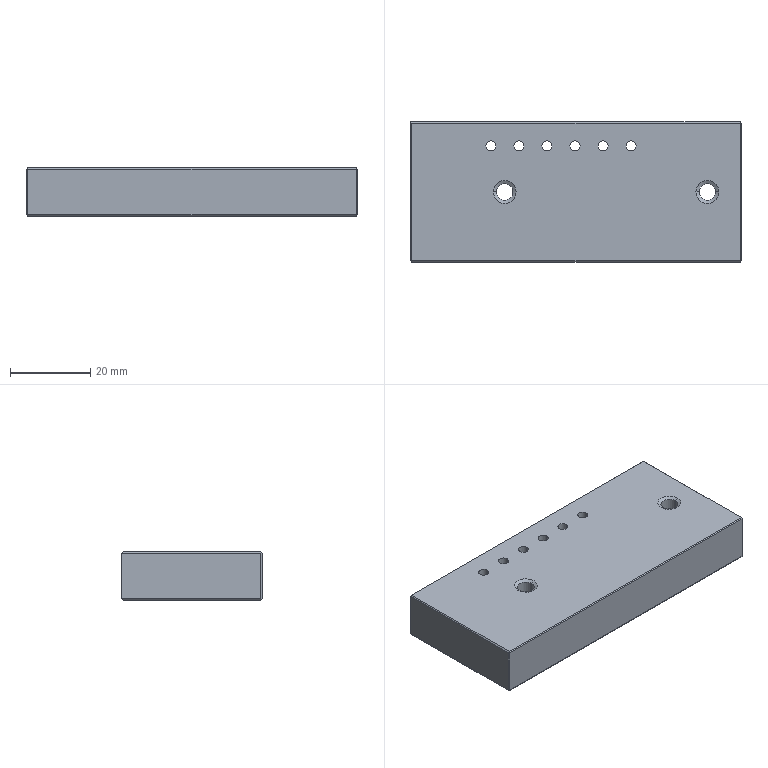Part | NX | 1 solid | 49 faces | box 82.5 x 35 x 12 mm | volume 33933 mm3 | plane 17 | cylinder 16 | cone 16 | commonest cylinder face diameters 2.5 x12 4.2 x4
STEP:
#1=CARTESIAN_POINT('',(-99.7,-60.,14.2));
#2=VERTEX_POINT('',#1);
#3=CARTESIAN_POINT('',(-99.7,-60.,2.8));
#4=VERTEX_POINT('',#3);
#5=CARTESIAN_POINT('',(-99.7,-60.,8.5));
#6=DIRECTION('',(0.,0.,-1.));
#7=VECTOR('',#6,1000.);
#8=LINE('',#5,#7);
#9=EDGE_CURVE('',#2,#4,#8,.T.);
#10=ORIENTED_EDGE('',*,*,#9,.T.);
#11=CARTESIAN_POINT('',(-17.8,-60.,2.8));
#12=VERTEX_POINT('',#11);
#13=CARTESIAN_POINT('',(0.,-60.,2.8));
#14=DIRECTION('',(-1.,0.,0.));
#15=VECTOR('',#14,1000.);
#16=LINE('',#13,#15);
#17=EDGE_CURVE('',#12,#4,#16,.T.);
#18=ORIENTED_EDGE('',*,*,#17,.F.);
#19=CARTESIAN_POINT('',(-17.8,-60.,14.2));
#20=VERTEX_POINT('',#19);
#21=CARTESIAN_POINT('',(-17.8,-60.,8.5));
#22=DIRECTION('',(0.,0.,1.));
#23=VECTOR('',#22,1000.);
#24=LINE('',#21,#23);
#25=EDGE_CURVE('',#12,#20,#24,.T.);
#26=ORIENTED_EDGE('',*,*,#25,.T.);
#27=CARTESIAN_POINT('',(0.,-60.,14.2));
#28=DIRECTION('',(1.,0.,0.));
#29=VECTOR('',#28,1000.);
#30=LINE('',#27,#29);
#31=EDGE_CURVE('',#2,#20,#30,.T.);
#32=ORIENTED_EDGE('',*,*,#31,.F.);
#33=EDGE_LOOP('',(#10,#18,#26,#32));
#34=FACE_BOUND('',#33,.T.);
#35=CARTESIAN_POINT('',(0.,-60.,0.));
#36=DIRECTION('',(0.,1.,0.));
#37=DIRECTION('',(1.,0.,0.));
#38=AXIS2_PLACEMENT_3D('',#35,#36,#37);
#39=PLANE('',#38);
#40=ADVANCED_FACE('',(#34),#39,.F.);
#41=CARTESIAN_POINT('',(-100.,-25.,2.8));
#42=VERTEX_POINT('',#41);
#43=CARTESIAN_POINT('',(-100.,-25.,14.2));
#44=VERTEX_POINT('',#43);
#45=CARTESIAN_POINT('',(-100.,-25.,0.));
#46=DIRECTION('',(0.,0.,1.));
#47=VECTOR('',#46,1000.);
#48=LINE('',#45,#47);
#49=EDGE_CURVE('',#42,#44,#48,.T.);
#50=ORIENTED_EDGE('',*,*,#49,.F.);
#51=CARTESIAN_POINT('',(-100.,-59.7,2.8));
#52=VERTEX_POINT('',#51);
#53=CARTESIAN_POINT('',(-100.,-42.5,2.8));
#54=DIRECTION('',(0.,1.,0.));
#55=VECTOR('',#54,1000.);
#56=LINE('',#53,#55);
#57=EDGE_CURVE('',#52,#42,#56,.T.);
#58=ORIENTED_EDGE('',*,*,#57,.F.);
#59=CARTESIAN_POINT('',(-100.,-59.7,14.2));
#60=VERTEX_POINT('',#59);
#61=CARTESIAN_POINT('',(-100.,-59.7,8.5));
#62=DIRECTION('',(0.,0.,-1.));
#63=VECTOR('',#62,1000.);
#64=LINE('',#61,#63);
#65=EDGE_CURVE('',#60,#52,#64,.T.);
#66=ORIENTED_EDGE('',*,*,#65,.F.);
#67=CARTESIAN_POINT('',(-100.,-42.5,14.2));
#68=DIRECTION('',(0.,-1.,0.));
#69=VECTOR('',#68,1000.);
#70=LINE('',#67,#69);
#71=EDGE_CURVE('',#44,#60,#70,.T.);
#72=ORIENTED_EDGE('',*,*,#71,.F.);
#73=EDGE_LOOP('',(#50,#58,#66,#72));
#74=FACE_BOUND('',#73,.T.);
#75=CARTESIAN_POINT('',(-100.,0.,0.));
#76=DIRECTION('',(1.,0.,0.));
#77=DIRECTION('',(0.,1.,0.));
#78=AXIS2_PLACEMENT_3D('',#75,#76,#77);
#79=PLANE('',#78);
#80=ADVANCED_FACE('',(#74),#79,.F.);
#81=CARTESIAN_POINT('',(-17.8,-25.,2.8));
#82=VERTEX_POINT('',#81);
#83=CARTESIAN_POINT('',(-17.8,-25.,14.2));
#84=VERTEX_POINT('',#83);
#85=CARTESIAN_POINT('',(-17.8,-25.,8.5));
#86=DIRECTION('',(0.,0.,1.));
#87=VECTOR('',#86,1000.);
#88=LINE('',#85,#87);
#89=EDGE_CURVE('',#82,#84,#88,.T.);
#90=ORIENTED_EDGE('',*,*,#89,.F.);
#91=CARTESIAN_POINT('',(0.,-25.,2.8));
#92=DIRECTION('',(1.,0.,0.));
#93=VECTOR('',#92,1000.);
#94=LINE('',#91,#93);
#95=EDGE_CURVE('',#42,#82,#94,.T.);
#96=ORIENTED_EDGE('',*,*,#95,.F.);
#97=ORIENTED_EDGE('',*,*,#49,.T.);
#98=CARTESIAN_POINT('',(0.,-25.,14.2));
#99=DIRECTION('',(1.,0.,0.));
#100=VECTOR('',#99,1000.);
#101=LINE('',#98,#100);
#102=EDGE_CURVE('',#44,#84,#101,.T.);
#103=ORIENTED_EDGE('',*,*,#102,.T.);
#104=EDGE_LOOP('',(#90,#96,#97,#103));
#105=FACE_BOUND('',#104,.T.);
#106=CARTESIAN_POINT('',(-8.5,-25.,1.2));
#107=DIRECTION('',(0.,-1.,0.));
#108=DIRECTION('',(-1.,0.,0.));
#109=AXIS2_PLACEMENT_3D('',#106,#107,#108);
#110=PLANE('',#109);
#111=ADVANCED_FACE('',(#105),#110,.F.);
#112=CARTESIAN_POINT('',(-17.8,-59.7,14.5));
#113=VERTEX_POINT('',#112);
#114=CARTESIAN_POINT('',(-99.7,-59.7,14.5));
#115=VERTEX_POINT('',#114);
#116=CARTESIAN_POINT('',(0.,-59.7,14.5));
#117=DIRECTION('',(-1.,0.,0.));
#118=VECTOR('',#117,1000.);
#119=LINE('',#116,#118);
#120=EDGE_CURVE('',#113,#115,#119,.T.);
#121=ORIENTED_EDGE('',*,*,#120,.T.);
#122=CARTESIAN_POINT('',(-99.85,-59.85,14.35));
#123=VERTEX_POINT('',#122);
#124=CARTESIAN_POINT('',(-114.2,-74.2,0.));
#125=DIRECTION('',(-0.5774,-0.5774,-0.5774));
#126=VECTOR('',#125,1000.);
#127=LINE('',#124,#126);
#128=EDGE_CURVE('',#115,#123,#127,.T.);
#129=ORIENTED_EDGE('',*,*,#128,.T.);
#130=CARTESIAN_POINT('',(-85.5,-74.2,0.));
#131=DIRECTION('',(0.5774,-0.5774,-0.5774));
#132=VECTOR('',#131,1000.);
#133=LINE('',#130,#132);
#134=EDGE_CURVE('',#123,#2,#133,.T.);
#135=ORIENTED_EDGE('',*,*,#134,.T.);
#136=ORIENTED_EDGE('',*,*,#31,.T.);
#137=CARTESIAN_POINT('',(-17.65,-59.85,14.35));
#138=VERTEX_POINT('',#137);
#139=CARTESIAN_POINT('',(-32.,-74.2,0.));
#140=DIRECTION('',(0.5774,0.5774,0.5774));
#141=VECTOR('',#140,1000.);
#142=LINE('',#139,#141);
#143=EDGE_CURVE('',#20,#138,#142,.T.);
#144=ORIENTED_EDGE('',*,*,#143,.T.);
#145=CARTESIAN_POINT('',(-3.3,-74.2,0.));
#146=DIRECTION('',(-0.5774,0.5774,0.5774));
#147=VECTOR('',#146,1000.);
#148=LINE('',#145,#147);
#149=EDGE_CURVE('',#138,#113,#148,.T.);
#150=ORIENTED_EDGE('',*,*,#149,.T.);
#151=EDGE_LOOP('',(#121,#129,#135,#136,#144,#150));
#152=FACE_BOUND('',#151,.T.);
#153=CARTESIAN_POINT('',(-51.25,-59.85,14.35));
#154=DIRECTION('',(0.,0.7071,-0.7071));
#155=DIRECTION('',(-1.,0.,0.));
#156=AXIS2_PLACEMENT_3D('',#153,#154,#155);
#157=PLANE('',#156);
#158=ADVANCED_FACE('',(#152),#157,.F.);
#159=CARTESIAN_POINT('',(-17.5,-25.3,14.2));
#160=VERTEX_POINT('',#159);
#161=CARTESIAN_POINT('',(-17.5,-59.7,14.2));
#162=VERTEX_POINT('',#161);
#163=CARTESIAN_POINT('',(-17.5,-42.5,14.2));
#164=DIRECTION('',(0.,-1.,0.));
#165=VECTOR('',#164,1000.);
#166=LINE('',#163,#165);
#167=EDGE_CURVE('',#160,#162,#166,.T.);
#168=ORIENTED_EDGE('',*,*,#167,.T.);
#169=CARTESIAN_POINT('',(-17.5,-59.7,2.8));
#170=VERTEX_POINT('',#169);
#171=CARTESIAN_POINT('',(-17.5,-59.7,8.5));
#172=DIRECTION('',(0.,0.,1.));
#173=VECTOR('',#172,1000.);
#174=LINE('',#171,#173);
#175=EDGE_CURVE('',#170,#162,#174,.T.);
#176=ORIENTED_EDGE('',*,*,#175,.F.);
#177=CARTESIAN_POINT('',(-17.5,-25.3,2.8));
#178=VERTEX_POINT('',#177);
#179=CARTESIAN_POINT('',(-17.5,-42.5,2.8));
#180=DIRECTION('',(0.,1.,0.));
#181=VECTOR('',#180,1000.);
#182=LINE('',#179,#181);
#183=EDGE_CURVE('',#170,#178,#182,.T.);
#184=ORIENTED_EDGE('',*,*,#183,.T.);
#185=CARTESIAN_POINT('',(-17.5,-25.3,8.5));
#186=DIRECTION('',(0.,0.,1.));
#187=VECTOR('',#186,1000.);
#188=LINE('',#185,#187);
#189=EDGE_CURVE('',#178,#160,#188,.T.);
#190=ORIENTED_EDGE('',*,*,#189,.T.);
#191=EDGE_LOOP('',(#168,#176,#184,#190));
#192=FACE_BOUND('',#191,.T.);
#193=CARTESIAN_POINT('',(-17.5,-38.5,5.));
#194=DIRECTION('',(1.,0.,0.));
#195=DIRECTION('',(0.,1.,0.));
#196=AXIS2_PLACEMENT_3D('',#193,#194,#195);
#197=PLANE('',#196);
#198=ADVANCED_FACE('',(#192),#197,.T.);
#199=CARTESIAN_POINT('',(-99.7,-25.3,14.5));
#200=VERTEX_POINT('',#199);
#201=CARTESIAN_POINT('',(-99.7,0.,14.5));
#202=DIRECTION('',(0.,-1.,0.));
#203=VECTOR('',#202,1000.);
#204=LINE('',#201,#203);
#205=EDGE_CURVE('',#200,#115,#204,.T.);
#206=ORIENTED_EDGE('',*,*,#205,.T.);
#207=ORIENTED_EDGE('',*,*,#120,.F.);
#208=CARTESIAN_POINT('',(-17.8,-25.3,14.5));
#209=VERTEX_POINT('',#208);
#210=CARTESIAN_POINT('',(-17.8,0.,14.5));
#211=DIRECTION('',(0.,1.,0.));
#212=VECTOR('',#211,1000.);
#213=LINE('',#210,#212);
#214=EDGE_CURVE('',#113,#209,#213,.T.);
#215=ORIENTED_EDGE('',*,*,#214,.T.);
#216=CARTESIAN_POINT('',(0.,-25.3,14.5));
#217=DIRECTION('',(1.,0.,0.));
#218=VECTOR('',#217,1000.);
#219=LINE('',#216,#218);
#220=EDGE_CURVE('',#200,#209,#219,.T.);
#221=ORIENTED_EDGE('',*,*,#220,.F.);
#222=EDGE_LOOP('',(#206,#207,#215,#221));
#223=FACE_BOUND('',#222,.T.);
#224=CARTESIAN_POINT('',(-28.797,-42.5,14.5));
#225=VERTEX_POINT('',#224);
#226=CARTESIAN_POINT('',(-23.077,-42.5,14.5));
#227=VERTEX_POINT('',#226);
#228=CARTESIAN_POINT('',(-25.937,-42.5,14.5));
#229=DIRECTION('',(0.,0.,1.));
#230=DIRECTION('',(1.,0.,0.));
#231=AXIS2_PLACEMENT_3D('',#228,#229,#230);
#232=CIRCLE('',#231,2.86);
#233=EDGE_CURVE('',#225,#227,#232,.T.);
#234=ORIENTED_EDGE('',*,*,#233,.F.);
#235=CARTESIAN_POINT('',(-25.937,-42.5,14.5));
#236=DIRECTION('',(0.,0.,1.));
#237=DIRECTION('',(1.,0.,0.));
#238=AXIS2_PLACEMENT_3D('',#235,#236,#237);
#239=CIRCLE('',#238,2.86);
#240=EDGE_CURVE('',#227,#225,#239,.T.);
#241=ORIENTED_EDGE('',*,*,#240,.F.);
#242=EDGE_LOOP('',(#234,#241));
#243=FACE_BOUND('',#242,.T.);
#244=CARTESIAN_POINT('',(-79.422,-42.5,14.5));
#245=VERTEX_POINT('',#244);
#246=CARTESIAN_POINT('',(-73.702,-42.5,14.5));
#247=VERTEX_POINT('',#246);
#248=CARTESIAN_POINT('',(-76.562,-42.5,14.5));
#249=DIRECTION('',(0.,0.,1.));
#250=DIRECTION('',(1.,0.,0.));
#251=AXIS2_PLACEMENT_3D('',#248,#249,#250);
#252=CIRCLE('',#251,2.86);
#253=EDGE_CURVE('',#245,#247,#252,.T.);
#254=ORIENTED_EDGE('',*,*,#253,.F.);
#255=CARTESIAN_POINT('',(-76.562,-42.5,14.5));
#256=DIRECTION('',(0.,0.,1.));
#257=DIRECTION('',(1.,0.,0.));
#258=AXIS2_PLACEMENT_3D('',#255,#256,#257);
#259=CIRCLE('',#258,2.86);
#260=EDGE_CURVE('',#247,#245,#259,.T.);
#261=ORIENTED_EDGE('',*,*,#260,.F.);
#262=EDGE_LOOP('',(#254,#261));
#263=FACE_BOUND('',#262,.T.);
#264=CARTESIAN_POINT('',(-43.75,-31.,14.5));
#265=VERTEX_POINT('',#264);
#266=CARTESIAN_POINT('',(-46.25,-31.,14.5));
#267=VERTEX_POINT('',#266);
#268=CARTESIAN_POINT('',(-45.,-31.,14.5));
#269=DIRECTION('',(0.,0.,-1.));
#270=DIRECTION('',(-1.,0.,0.));
#271=AXIS2_PLACEMENT_3D('',#268,#269,#270);
#272=CIRCLE('',#271,1.25);
#273=EDGE_CURVE('',#265,#267,#272,.T.);
#274=ORIENTED_EDGE('',*,*,#273,.T.);
#275=CARTESIAN_POINT('',(-45.,-31.,14.5));
#276=DIRECTION('',(0.,0.,-1.));
#277=DIRECTION('',(-1.,0.,0.));
#278=AXIS2_PLACEMENT_3D('',#275,#276,#277);
#279=CIRCLE('',#278,1.25);
#280=EDGE_CURVE('',#267,#265,#279,.T.);
#281=ORIENTED_EDGE('',*,*,#280,.T.);
#282=EDGE_LOOP('',(#274,#281));
#283=FACE_BOUND('',#282,.T.);
#284=CARTESIAN_POINT('',(-50.75,-31.,14.5));
#285=VERTEX_POINT('',#284);
#286=CARTESIAN_POINT('',(-53.25,-31.,14.5));
#287=VERTEX_POINT('',#286);
#288=CARTESIAN_POINT('',(-52.,-31.,14.5));
#289=DIRECTION('',(0.,0.,-1.));
#290=DIRECTION('',(-1.,0.,0.));
#291=AXIS2_PLACEMENT_3D('',#288,#289,#290);
#292=CIRCLE('',#291,1.25);
#293=EDGE_CURVE('',#285,#287,#292,.T.);
#294=ORIENTED_EDGE('',*,*,#293,.T.);
#295=CARTESIAN_POINT('',(-52.,-31.,14.5));
#296=DIRECTION('',(0.,0.,-1.));
#297=DIRECTION('',(-1.,0.,0.));
#298=AXIS2_PLACEMENT_3D('',#295,#296,#297);
#299=CIRCLE('',#298,1.25);
#300=EDGE_CURVE('',#287,#285,#299,.T.);
#301=ORIENTED_EDGE('',*,*,#300,.T.);
#302=EDGE_LOOP('',(#294,#301));
#303=FACE_BOUND('',#302,.T.);
#304=CARTESIAN_POINT('',(-57.75,-31.,14.5));
#305=VERTEX_POINT('',#304);
#306=CARTESIAN_POINT('',(-60.25,-31.,14.5));
#307=VERTEX_POINT('',#306);
#308=CARTESIAN_POINT('',(-59.,-31.,14.5));
#309=DIRECTION('',(0.,0.,-1.));
#310=DIRECTION('',(-1.,0.,0.));
#311=AXIS2_PLACEMENT_3D('',#308,#309,#310);
#312=CIRCLE('',#311,1.25);
#313=EDGE_CURVE('',#305,#307,#312,.T.);
#314=ORIENTED_EDGE('',*,*,#313,.T.);
#315=CARTESIAN_POINT('',(-59.,-31.,14.5));
#316=DIRECTION('',(0.,0.,-1.));
#317=DIRECTION('',(-1.,0.,0.));
#318=AXIS2_PLACEMENT_3D('',#315,#316,#317);
#319=CIRCLE('',#318,1.25);
#320=EDGE_CURVE('',#307,#305,#319,.T.);
#321=ORIENTED_EDGE('',*,*,#320,.T.);
#322=EDGE_LOOP('',(#314,#321));
#323=FACE_BOUND('',#322,.T.);
#324=CARTESIAN_POINT('',(-64.75,-31.,14.5));
#325=VERTEX_POINT('',#324);
#326=CARTESIAN_POINT('',(-67.25,-31.,14.5));
#327=VERTEX_POINT('',#326);
#328=CARTESIAN_POINT('',(-66.,-31.,14.5));
#329=DIRECTION('',(0.,0.,-1.));
#330=DIRECTION('',(-1.,0.,0.));
#331=AXIS2_PLACEMENT_3D('',#328,#329,#330);
#332=CIRCLE('',#331,1.25);
#333=EDGE_CURVE('',#325,#327,#332,.T.);
#334=ORIENTED_EDGE('',*,*,#333,.T.);
#335=CARTESIAN_POINT('',(-66.,-31.,14.5));
#336=DIRECTION('',(0.,0.,-1.));
#337=DIRECTION('',(-1.,0.,0.));
#338=AXIS2_PLACEMENT_3D('',#335,#336,#337);
#339=CIRCLE('',#338,1.25);
#340=EDGE_CURVE('',#327,#325,#339,.T.);
#341=ORIENTED_EDGE('',*,*,#340,.T.);
#342=EDGE_LOOP('',(#334,#341));
#343=FACE_BOUND('',#342,.T.);
#344=CARTESIAN_POINT('',(-71.75,-31.,14.5));
#345=VERTEX_POINT('',#344);
#346=CARTESIAN_POINT('',(-74.25,-31.,14.5));
#347=VERTEX_POINT('',#346);
#348=CARTESIAN_POINT('',(-73.,-31.,14.5));
#349=DIRECTION('',(0.,0.,-1.));
#350=DIRECTION('',(-1.,0.,0.));
#351=AXIS2_PLACEMENT_3D('',#348,#349,#350);
#352=CIRCLE('',#351,1.25);
#353=EDGE_CURVE('',#345,#347,#352,.T.);
#354=ORIENTED_EDGE('',*,*,#353,.T.);
#355=CARTESIAN_POINT('',(-73.,-31.,14.5));
#356=DIRECTION('',(0.,0.,-1.));
#357=DIRECTION('',(-1.,0.,0.));
#358=AXIS2_PLACEMENT_3D('',#355,#356,#357);
#359=CIRCLE('',#358,1.25);
#360=EDGE_CURVE('',#347,#345,#359,.T.);
#361=ORIENTED_EDGE('',*,*,#360,.T.);
#362=EDGE_LOOP('',(#354,#361));
#363=FACE_BOUND('',#362,.T.);
#364=CARTESIAN_POINT('',(-78.75,-31.,14.5));
#365=VERTEX_POINT('',#364);
#366=CARTESIAN_POINT('',(-81.25,-31.,14.5));
#367=VERTEX_POINT('',#366);
#368=CARTESIAN_POINT('',(-80.,-31.,14.5));
#369=DIRECTION('',(0.,0.,-1.));
#370=DIRECTION('',(-1.,0.,0.));
#371=AXIS2_PLACEMENT_3D('',#368,#369,#370);
#372=CIRCLE('',#371,1.25);
#373=EDGE_CURVE('',#365,#367,#372,.T.);
#374=ORIENTED_EDGE('',*,*,#373,.T.);
#375=CARTESIAN_POINT('',(-80.,-31.,14.5));
#376=DIRECTION('',(0.,0.,-1.));
#377=DIRECTION('',(-1.,0.,0.));
#378=AXIS2_PLACEMENT_3D('',#375,#376,#377);
#379=CIRCLE('',#378,1.25);
#380=EDGE_CURVE('',#367,#365,#379,.T.);
#381=ORIENTED_EDGE('',*,*,#380,.T.);
#382=EDGE_LOOP('',(#374,#381));
#383=FACE_BOUND('',#382,.T.);
#384=CARTESIAN_POINT('',(-20.5,7.5,14.5));
#385=DIRECTION('',(0.,0.,-1.));
#386=DIRECTION('',(0.,-1.,0.));
#387=AXIS2_PLACEMENT_3D('',#384,#385,#386);
#388=PLANE('',#387);
#389=ADVANCED_FACE('',(#223,#243,#263,#283,#303,#323,#343,#363,#383),#388,.F.);
#390=ORIENTED_EDGE('',*,*,#9,.F.);
#391=ORIENTED_EDGE('',*,*,#134,.F.);
#392=CARTESIAN_POINT('',(-114.2,-45.5,0.));
#393=DIRECTION('',(0.5774,-0.5774,0.5774));
#394=VECTOR('',#393,1000.);
#395=LINE('',#392,#394);
#396=EDGE_CURVE('',#60,#123,#395,.T.);
#397=ORIENTED_EDGE('',*,*,#396,.F.);
#398=ORIENTED_EDGE('',*,*,#65,.T.);
#399=CARTESIAN_POINT('',(-99.85,-59.85,2.65));
#400=VERTEX_POINT('',#399);
#401=CARTESIAN_POINT('',(-97.2,-62.5,0.));
#402=DIRECTION('',(0.5774,-0.5774,-0.5774));
#403=VECTOR('',#402,1000.);
#404=LINE('',#401,#403);
#405=EDGE_CURVE('',#52,#400,#404,.T.);
#406=ORIENTED_EDGE('',*,*,#405,.T.);
#407=CARTESIAN_POINT('',(-102.5,-57.2,0.));
#408=DIRECTION('',(-0.5774,0.5774,-0.5774));
#409=VECTOR('',#408,1000.);
#410=LINE('',#407,#409);
#411=EDGE_CURVE('',#4,#400,#410,.T.);
#412=ORIENTED_EDGE('',*,*,#411,.F.);
#413=EDGE_LOOP('',(#390,#391,#397,#398,#406,#412));
#414=FACE_BOUND('',#413,.T.);
#415=CARTESIAN_POINT('',(-99.85,-59.85,8.5));
#416=DIRECTION('',(-0.7071,-0.7071,0.));
#417=DIRECTION('',(-0.7071,0.7071,0.));
#418=AXIS2_PLACEMENT_3D('',#415,#416,#417);
#419=PLANE('',#418);
#420=ADVANCED_FACE('',(#414),#419,.T.);
#421=CARTESIAN_POINT('',(-17.8,-59.7,2.5));
#422=VERTEX_POINT('',#421);
#423=CARTESIAN_POINT('',(-17.8,-25.3,2.5));
#424=VERTEX_POINT('',#423);
#425=CARTESIAN_POINT('',(-17.8,0.,2.5));
#426=DIRECTION('',(0.,1.,0.));
#427=VECTOR('',#426,1000.);
#428=LINE('',#425,#427);
#429=EDGE_CURVE('',#422,#424,#428,.T.);
#430=ORIENTED_EDGE('',*,*,#429,.T.);
#431=CARTESIAN_POINT('',(-17.65,-25.15,2.65));
#432=VERTEX_POINT('',#431);
#433=CARTESIAN_POINT('',(0.,-7.5,20.3));
#434=DIRECTION('',(-0.5774,-0.5774,-0.5774));
#435=VECTOR('',#434,1000.);
#436=LINE('',#433,#435);
#437=EDGE_CURVE('',#432,#424,#436,.T.);
#438=ORIENTED_EDGE('',*,*,#437,.F.);
#439=CARTESIAN_POINT('',(-42.8,0.,-22.5));
#440=DIRECTION('',(0.5774,-0.5774,0.5774));
#441=VECTOR('',#440,1000.);
#442=LINE('',#439,#441);
#443=EDGE_CURVE('',#432,#178,#442,.T.);
#444=ORIENTED_EDGE('',*,*,#443,.T.);
#445=ORIENTED_EDGE('',*,*,#183,.F.);
#446=CARTESIAN_POINT('',(-17.65,-59.85,2.65));
#447=VERTEX_POINT('',#446);
#448=CARTESIAN_POINT('',(0.,-42.2,20.3));
#449=DIRECTION('',(0.5774,0.5774,0.5774));
#450=VECTOR('',#449,1000.);
#451=LINE('',#448,#450);
#452=EDGE_CURVE('',#447,#170,#451,.T.);
#453=ORIENTED_EDGE('',*,*,#452,.F.);
#454=CARTESIAN_POINT('',(0.,-77.5,20.3));
#455=DIRECTION('',(-0.5774,0.5774,-0.5774));
#456=VECTOR('',#455,1000.);
#457=LINE('',#454,#456);
#458=EDGE_CURVE('',#447,#422,#457,.T.);
#459=ORIENTED_EDGE('',*,*,#458,.T.);
#460=EDGE_LOOP('',(#430,#438,#444,#445,#453,#459));
#461=FACE_BOUND('',#460,.T.);
#462=CARTESIAN_POINT('',(-17.65,-42.5,2.65));
#463=DIRECTION('',(-0.7071,0.,0.7071));
#464=DIRECTION('',(0.,1.,0.));
#465=AXIS2_PLACEMENT_3D('',#462,#463,#464);
#466=PLANE('',#465);
#467=ADVANCED_FACE('',(#461),#466,.F.);
#468=CARTESIAN_POINT('',(-99.7,-25.3,2.5));
#469=VERTEX_POINT('',#468);
#470=CARTESIAN_POINT('',(0.,-25.3,2.5));
#471=DIRECTION('',(1.,0.,0.));
#472=VECTOR('',#471,1000.);
#473=LINE('',#470,#472);
#474=EDGE_CURVE('',#469,#424,#473,.T.);
#475=ORIENTED_EDGE('',*,*,#474,.T.);
#476=ORIENTED_EDGE('',*,*,#429,.F.);
#477=CARTESIAN_POINT('',(-99.7,-59.7,2.5));
#478=VERTEX_POINT('',#477);
#479=CARTESIAN_POINT('',(0.,-59.7,2.5));
#480=DIRECTION('',(1.,0.,0.));
#481=VECTOR('',#480,1000.);
#482=LINE('',#479,#481);
#483=EDGE_CURVE('',#478,#422,#482,.T.);
#484=ORIENTED_EDGE('',*,*,#483,.F.);
#485=CARTESIAN_POINT('',(-99.7,0.,2.5));
#486=DIRECTION('',(0.,1.,0.));
#487=VECTOR('',#486,1000.);
#488=LINE('',#485,#487);
#489=EDGE_CURVE('',#478,#469,#488,.T.);
#490=ORIENTED_EDGE('',*,*,#489,.T.);
#491=EDGE_LOOP('',(#475,#476,#484,#490));
#492=FACE_BOUND('',#491,.T.);
#493=CARTESIAN_POINT('',(-28.037,-42.5,2.5));
#494=VERTEX_POINT('',#493);
#495=CARTESIAN_POINT('',(-23.837,-42.5,2.5));
#496=VERTEX_POINT('',#495);
#497=CARTESIAN_POINT('',(-25.937,-42.5,2.5));
#498=DIRECTION('',(0.,0.,1.));
#499=DIRECTION('',(1.,0.,0.));
#500=AXIS2_PLACEMENT_3D('',#497,#498,#499);
#501=CIRCLE('',#500,2.1);
#502=EDGE_CURVE('',#494,#496,#501,.T.);
#503=ORIENTED_EDGE('',*,*,#502,.T.);
#504=CARTESIAN_POINT('',(-25.937,-42.5,2.5));
#505=DIRECTION('',(0.,0.,1.));
#506=DIRECTION('',(1.,0.,0.));
#507=AXIS2_PLACEMENT_3D('',#504,#505,#506);
#508=CIRCLE('',#507,2.1);
#509=EDGE_CURVE('',#496,#494,#508,.T.);
#510=ORIENTED_EDGE('',*,*,#509,.T.);
#511=EDGE_LOOP('',(#503,#510));
#512=FACE_BOUND('',#511,.T.);
#513=CARTESIAN_POINT('',(-78.3,-31.,2.5));
#514=VERTEX_POINT('',#513);
#515=CARTESIAN_POINT('',(-81.7,-31.,2.5));
#516=VERTEX_POINT('',#515);
#517=CARTESIAN_POINT('',(-80.,-31.,2.5));
#518=DIRECTION('',(0.,0.,-1.));
#519=DIRECTION('',(-1.,0.,0.));
#520=AXIS2_PLACEMENT_3D('',#517,#518,#519);
#521=CIRCLE('',#520,1.7);
#522=EDGE_CURVE('',#514,#516,#521,.T.);
#523=ORIENTED_EDGE('',*,*,#522,.F.);
#524=CARTESIAN_POINT('',(-80.,-31.,2.5));
#525=DIRECTION('',(0.,0.,-1.));
#526=DIRECTION('',(-1.,0.,0.));
#527=AXIS2_PLACEMENT_3D('',#524,#525,#526);
#528=CIRCLE('',#527,1.7);
#529=EDGE_CURVE('',#516,#514,#528,.T.);
#530=ORIENTED_EDGE('',*,*,#529,.F.);
#531=EDGE_LOOP('',(#523,#530));
#532=FACE_BOUND('',#531,.T.);
#533=CARTESIAN_POINT('',(-64.3,-31.,2.5));
#534=VERTEX_POINT('',#533);
#535=CARTESIAN_POINT('',(-67.7,-31.,2.5));
#536=VERTEX_POINT('',#535);
#537=CARTESIAN_POINT('',(-66.,-31.,2.5));
#538=DIRECTION('',(0.,0.,-1.));
#539=DIRECTION('',(-1.,0.,0.));
#540=AXIS2_PLACEMENT_3D('',#537,#538,#539);
#541=CIRCLE('',#540,1.7);
#542=EDGE_CURVE('',#534,#536,#541,.T.);
#543=ORIENTED_EDGE('',*,*,#542,.F.);
#544=CARTESIAN_POINT('',(-66.,-31.,2.5));
#545=DIRECTION('',(0.,0.,-1.));
#546=DIRECTION('',(-1.,0.,0.));
#547=AXIS2_PLACEMENT_3D('',#544,#545,#546);
#548=CIRCLE('',#547,1.7);
#549=EDGE_CURVE('',#536,#534,#548,.T.);
#550=ORIENTED_EDGE('',*,*,#549,.F.);
#551=EDGE_LOOP('',(#543,#550));
#552=FACE_BOUND('',#551,.T.);
#553=CARTESIAN_POINT('',(-50.3,-31.,2.5));
#554=VERTEX_POINT('',#553);
#555=CARTESIAN_POINT('',(-53.7,-31.,2.5));
#556=VERTEX_POINT('',#555);
#557=CARTESIAN_POINT('',(-52.,-31.,2.5));
#558=DIRECTION('',(0.,0.,-1.));
#559=DIRECTION('',(-1.,0.,0.));
#560=AXIS2_PLACEMENT_3D('',#557,#558,#559);
#561=CIRCLE('',#560,1.7);
#562=EDGE_CURVE('',#554,#556,#561,.T.);
#563=ORIENTED_EDGE('',*,*,#562,.F.);
#564=CARTESIAN_POINT('',(-52.,-31.,2.5));
#565=DIRECTION('',(0.,0.,-1.));
#566=DIRECTION('',(-1.,0.,0.));
#567=AXIS2_PLACEMENT_3D('',#564,#565,#566);
#568=CIRCLE('',#567,1.7);
#569=EDGE_CURVE('',#556,#554,#568,.T.);
#570=ORIENTED_EDGE('',*,*,#569,.F.);
#571=EDGE_LOOP('',(#563,#570));
#572=FACE_BOUND('',#571,.T.);
#573=CARTESIAN_POINT('',(-78.662,-42.5,2.5));
#574=VERTEX_POINT('',#573);
#575=CARTESIAN_POINT('',(-74.462,-42.5,2.5));
#576=VERTEX_POINT('',#575);
#577=CARTESIAN_POINT('',(-76.562,-42.5,2.5));
#578=DIRECTION('',(0.,0.,1.));
#579=DIRECTION('',(1.,0.,0.));
#580=AXIS2_PLACEMENT_3D('',#577,#578,#579);
#581=CIRCLE('',#580,2.1);
#582=EDGE_CURVE('',#574,#576,#581,.T.);
#583=ORIENTED_EDGE('',*,*,#582,.T.);
#584=CARTESIAN_POINT('',(-76.562,-42.5,2.5));
#585=DIRECTION('',(0.,0.,1.));
#586=DIRECTION('',(1.,0.,0.));
#587=AXIS2_PLACEMENT_3D('',#584,#585,#586);
#588=CIRCLE('',#587,2.1);
#589=EDGE_CURVE('',#576,#574,#588,.T.);
#590=ORIENTED_EDGE('',*,*,#589,.T.);
#591=EDGE_LOOP('',(#583,#590));
#592=FACE_BOUND('',#591,.T.);
#593=CARTESIAN_POINT('',(-43.3,-31.,2.5));
#594=VERTEX_POINT('',#593);
#595=CARTESIAN_POINT('',(-46.7,-31.,2.5));
#596=VERTEX_POINT('',#595);
#597=CARTESIAN_POINT('',(-45.,-31.,2.5));
#598=DIRECTION('',(0.,0.,-1.));
#599=DIRECTION('',(-1.,0.,0.));
#600=AXIS2_PLACEMENT_3D('',#597,#598,#599);
#601=CIRCLE('',#600,1.7);
#602=EDGE_CURVE('',#594,#596,#601,.T.);
#603=ORIENTED_EDGE('',*,*,#602,.F.);
#604=CARTESIAN_POINT('',(-45.,-31.,2.5));
#605=DIRECTION('',(0.,0.,-1.));
#606=DIRECTION('',(-1.,0.,0.));
#607=AXIS2_PLACEMENT_3D('',#604,#605,#606);
#608=CIRCLE('',#607,1.7);
#609=EDGE_CURVE('',#596,#594,#608,.T.);
#610=ORIENTED_EDGE('',*,*,#609,.F.);
#611=EDGE_LOOP('',(#603,#610));
#612=FACE_BOUND('',#611,.T.);
#613=CARTESIAN_POINT('',(-57.3,-31.,2.5));
#614=VERTEX_POINT('',#613);
#615=CARTESIAN_POINT('',(-60.7,-31.,2.5));
#616=VERTEX_POINT('',#615);
#617=CARTESIAN_POINT('',(-59.,-31.,2.5));
#618=DIRECTION('',(0.,0.,-1.));
#619=DIRECTION('',(-1.,0.,0.));
#620=AXIS2_PLACEMENT_3D('',#617,#618,#619);
#621=CIRCLE('',#620,1.7);
#622=EDGE_CURVE('',#614,#616,#621,.T.);
#623=ORIENTED_EDGE('',*,*,#622,.F.);
#624=CARTESIAN_POINT('',(-59.,-31.,2.5));
#625=DIRECTION('',(0.,0.,-1.));
#626=DIRECTION('',(-1.,0.,0.));
#627=AXIS2_PLACEMENT_3D('',#624,#625,#626);
#628=CIRCLE('',#627,1.7);
#629=EDGE_CURVE('',#616,#614,#628,.T.);
#630=ORIENTED_EDGE('',*,*,#629,.F.);
#631=EDGE_LOOP('',(#623,#630));
#632=FACE_BOUND('',#631,.T.);
#633=CARTESIAN_POINT('',(-71.3,-31.,2.5));
#634=VERTEX_POINT('',#633);
#635=CARTESIAN_POINT('',(-74.7,-31.,2.5));
#636=VERTEX_POINT('',#635);
#637=CARTESIAN_POINT('',(-73.,-31.,2.5));
#638=DIRECTION('',(0.,0.,-1.));
#639=DIRECTION('',(-1.,0.,0.));
#640=AXIS2_PLACEMENT_3D('',#637,#638,#639);
#641=CIRCLE('',#640,1.7);
#642=EDGE_CURVE('',#634,#636,#641,.T.);
#643=ORIENTED_EDGE('',*,*,#642,.F.);
#644=CARTESIAN_POINT('',(-73.,-31.,2.5));
#645=DIRECTION('',(0.,0.,-1.));
#646=DIRECTION('',(-1.,0.,0.));
#647=AXIS2_PLACEMENT_3D('',#644,#645,#646);
#648=CIRCLE('',#647,1.7);
#649=EDGE_CURVE('',#636,#634,#648,.T.);
#650=ORIENTED_EDGE('',*,*,#649,.F.);
#651=EDGE_LOOP('',(#643,#650));
#652=FACE_BOUND('',#651,.T.);
#653=CARTESIAN_POINT('',(-35.,0.,2.5));
#654=DIRECTION('',(0.,0.,1.));
#655=DIRECTION('',(1.,0.,0.));
#656=AXIS2_PLACEMENT_3D('',#653,#654,#655);
#657=PLANE('',#656);
#658=ADVANCED_FACE('',(#492,#512,#532,#552,#572,#592,#612,#632,#652),#657,.F.);
#659=ORIENTED_EDGE('',*,*,#17,.T.);
#660=ORIENTED_EDGE('',*,*,#411,.T.);
#661=CARTESIAN_POINT('',(-97.2,-57.2,0.));
#662=DIRECTION('',(0.5774,0.5774,-0.5774));
#663=VECTOR('',#662,1000.);
#664=LINE('',#661,#663);
#665=EDGE_CURVE('',#400,#478,#664,.T.);
#666=ORIENTED_EDGE('',*,*,#665,.T.);
#667=ORIENTED_EDGE('',*,*,#483,.T.);
#668=ORIENTED_EDGE('',*,*,#458,.F.);
#669=CARTESIAN_POINT('',(0.,-42.2,-15.));
#670=DIRECTION('',(-0.5774,-0.5774,0.5774));
#671=VECTOR('',#670,1000.);
#672=LINE('',#669,#671);
#673=EDGE_CURVE('',#447,#12,#672,.T.);
#674=ORIENTED_EDGE('',*,*,#673,.T.);
#675=EDGE_LOOP('',(#659,#660,#666,#667,#668,#674));
#676=FACE_BOUND('',#675,.T.);
#677=CARTESIAN_POINT('',(-51.25,-59.85,2.65));
#678=DIRECTION('',(0.,0.7071,0.7071));
#679=DIRECTION('',(1.,0.,0.));
#680=AXIS2_PLACEMENT_3D('',#677,#678,#679);
#681=PLANE('',#680);
#682=ADVANCED_FACE('',(#676),#681,.F.);
#683=ORIENTED_EDGE('',*,*,#25,.F.);
#684=ORIENTED_EDGE('',*,*,#673,.F.);
#685=ORIENTED_EDGE('',*,*,#452,.T.);
#686=ORIENTED_EDGE('',*,*,#175,.T.);
#687=CARTESIAN_POINT('',(0.,-42.2,-3.3));
#688=DIRECTION('',(0.5774,0.5774,-0.5774));
#689=VECTOR('',#688,1000.);
#690=LINE('',#687,#689);
#691=EDGE_CURVE('',#138,#162,#690,.T.);
#692=ORIENTED_EDGE('',*,*,#691,.F.);
#693=ORIENTED_EDGE('',*,*,#143,.F.);
#694=EDGE_LOOP('',(#683,#684,#685,#686,#692,#693));
#695=FACE_BOUND('',#694,.T.);
#696=CARTESIAN_POINT('',(-17.65,-59.85,8.5));
#697=DIRECTION('',(0.7071,-0.7071,0.));
#698=DIRECTION('',(0.,0.,-1.));
#699=AXIS2_PLACEMENT_3D('',#696,#697,#698);
#700=PLANE('',#699);
#701=ADVANCED_FACE('',(#695),#700,.T.);
#702=ORIENTED_EDGE('',*,*,#489,.F.);
#703=ORIENTED_EDGE('',*,*,#665,.F.);
#704=ORIENTED_EDGE('',*,*,#405,.F.);
#705=ORIENTED_EDGE('',*,*,#57,.T.);
#706=CARTESIAN_POINT('',(-125.,0.,27.8));
#707=DIRECTION('',(0.5774,-0.5774,-0.5774));
#708=VECTOR('',#707,1000.);
#709=LINE('',#706,#708);
#710=EDGE_CURVE('',#42,#469,#709,.T.);
#711=ORIENTED_EDGE('',*,*,#710,.T.);
#712=EDGE_LOOP('',(#702,#703,#704,#705,#711));
#713=FACE_BOUND('',#712,.T.);
#714=CARTESIAN_POINT('',(-99.85,-42.5,2.65));
#715=DIRECTION('',(-0.7071,0.,-0.7071));
#716=DIRECTION('',(-0.7071,0.,0.7071));
#717=AXIS2_PLACEMENT_3D('',#714,#715,#716);
#718=PLANE('',#717);
#719=ADVANCED_FACE('',(#713),#718,.T.);
#720=ORIENTED_EDGE('',*,*,#102,.F.);
#721=CARTESIAN_POINT('',(-125.,0.,-10.8));
#722=DIRECTION('',(0.5774,-0.5774,0.5774));
#723=VECTOR('',#722,1000.);
#724=LINE('',#721,#723);
#725=EDGE_CURVE('',#44,#200,#724,.T.);
#726=ORIENTED_EDGE('',*,*,#725,.T.);
#727=ORIENTED_EDGE('',*,*,#220,.T.);
#728=CARTESIAN_POINT('',(-17.65,-25.15,14.35));
#729=VERTEX_POINT('',#728);
#730=CARTESIAN_POINT('',(-3.3,-10.8,0.));
#731=DIRECTION('',(0.5774,0.5774,-0.5774));
#732=VECTOR('',#731,1000.);
#733=LINE('',#730,#732);
#734=EDGE_CURVE('',#209,#729,#733,.T.);
#735=ORIENTED_EDGE('',*,*,#734,.T.);
#736=CARTESIAN_POINT('',(-42.8,0.,-10.8));
#737=DIRECTION('',(0.5774,-0.5774,0.5774));
#738=VECTOR('',#737,1000.);
#739=LINE('',#736,#738);
#740=EDGE_CURVE('',#84,#729,#739,.T.);
#741=ORIENTED_EDGE('',*,*,#740,.F.);
#742=EDGE_LOOP('',(#720,#726,#727,#735,#741));
#743=FACE_BOUND('',#742,.T.);
#744=CARTESIAN_POINT('',(-51.25,-25.15,14.35));
#745=DIRECTION('',(0.,-0.7071,-0.7071));
#746=DIRECTION('',(0.,-0.7071,0.7071));
#747=AXIS2_PLACEMENT_3D('',#744,#745,#746);
#748=PLANE('',#747);
#749=ADVANCED_FACE('',(#743),#748,.F.);
#750=ORIENTED_EDGE('',*,*,#167,.F.);
#751=CARTESIAN_POINT('',(-42.8,0.,39.5));
#752=DIRECTION('',(-0.5774,0.5774,0.5774));
#753=VECTOR('',#752,1000.);
#754=LINE('',#751,#753);
#755=EDGE_CURVE('',#160,#729,#754,.T.);
#756=ORIENTED_EDGE('',*,*,#755,.T.);
#757=ORIENTED_EDGE('',*,*,#734,.F.);
#758=ORIENTED_EDGE('',*,*,#214,.F.);
#759=ORIENTED_EDGE('',*,*,#149,.F.);
#760=ORIENTED_EDGE('',*,*,#691,.T.);
#761=EDGE_LOOP('',(#750,#756,#757,#758,#759,#760));
#762=FACE_BOUND('',#761,.T.);
#763=CARTESIAN_POINT('',(-17.65,-42.5,14.35));
#764=DIRECTION('',(0.7071,0.,0.7071));
#765=DIRECTION('',(0.,-1.,0.));
#766=AXIS2_PLACEMENT_3D('',#763,#764,#765);
#767=PLANE('',#766);
#768=ADVANCED_FACE('',(#762),#767,.T.);
#769=ORIENTED_EDGE('',*,*,#89,.T.);
#770=ORIENTED_EDGE('',*,*,#740,.T.);
#771=ORIENTED_EDGE('',*,*,#755,.F.);
#772=ORIENTED_EDGE('',*,*,#189,.F.);
#773=ORIENTED_EDGE('',*,*,#443,.F.);
#774=CARTESIAN_POINT('',(-42.8,0.,27.8));
#775=DIRECTION('',(0.5774,-0.5774,-0.5774));
#776=VECTOR('',#775,1000.);
#777=LINE('',#774,#776);
#778=EDGE_CURVE('',#82,#432,#777,.T.);
#779=ORIENTED_EDGE('',*,*,#778,.F.);
#780=EDGE_LOOP('',(#769,#770,#771,#772,#773,#779));
#781=FACE_BOUND('',#780,.T.);
#782=CARTESIAN_POINT('',(-17.65,-25.15,8.5));
#783=DIRECTION('',(-0.7071,-0.7071,0.));
#784=DIRECTION('',(-0.7071,0.7071,0.));
#785=AXIS2_PLACEMENT_3D('',#782,#783,#784);
#786=PLANE('',#785);
#787=ADVANCED_FACE('',(#781),#786,.F.);
#788=ORIENTED_EDGE('',*,*,#205,.F.);
#789=ORIENTED_EDGE('',*,*,#725,.F.);
#790=ORIENTED_EDGE('',*,*,#71,.T.);
#791=ORIENTED_EDGE('',*,*,#396,.T.);
#792=ORIENTED_EDGE('',*,*,#128,.F.);
#793=EDGE_LOOP('',(#788,#789,#790,#791,#792));
#794=FACE_BOUND('',#793,.T.);
#795=CARTESIAN_POINT('',(-99.85,-42.5,14.35));
#796=DIRECTION('',(-0.7071,0.,0.7071));
#797=DIRECTION('',(0.,1.,0.));
#798=AXIS2_PLACEMENT_3D('',#795,#796,#797);
#799=PLANE('',#798);
#800=ADVANCED_FACE('',(#794),#799,.T.);
#801=ORIENTED_EDGE('',*,*,#710,.F.);
#802=ORIENTED_EDGE('',*,*,#95,.T.);
#803=ORIENTED_EDGE('',*,*,#778,.T.);
#804=ORIENTED_EDGE('',*,*,#437,.T.);
#805=ORIENTED_EDGE('',*,*,#474,.F.);
#806=EDGE_LOOP('',(#801,#802,#803,#804,#805));
#807=FACE_BOUND('',#806,.T.);
#808=CARTESIAN_POINT('',(-51.25,-25.15,2.65));
#809=DIRECTION('',(0.,0.7071,-0.7071));
#810=DIRECTION('',(-1.,0.,0.));
#811=AXIS2_PLACEMENT_3D('',#808,#809,#810);
#812=PLANE('',#811);
#813=ADVANCED_FACE('',(#807),#812,.T.);
#814=CARTESIAN_POINT('',(-28.037,-42.5,14.061));
#815=VERTEX_POINT('',#814);
#816=CARTESIAN_POINT('',(-23.837,-42.5,14.061));
#817=VERTEX_POINT('',#816);
#818=CARTESIAN_POINT('',(-25.937,-42.5,14.061));
#819=DIRECTION('',(0.,0.,1.));
#820=DIRECTION('',(1.,0.,0.));
#821=AXIS2_PLACEMENT_3D('',#818,#819,#820);
#822=CIRCLE('',#821,2.1);
#823=EDGE_CURVE('',#815,#817,#822,.T.);
#824=ORIENTED_EDGE('',*,*,#823,.T.);
#825=CARTESIAN_POINT('',(-23.837,-42.5,14.5));
#826=DIRECTION('',(0.,0.,1.));
#827=VECTOR('',#826,1000.);
#828=LINE('',#825,#827);
#829=EDGE_CURVE('',#496,#817,#828,.T.);
#830=ORIENTED_EDGE('',*,*,#829,.F.);
#831=ORIENTED_EDGE('',*,*,#502,.F.);
#832=CARTESIAN_POINT('',(-28.037,-42.5,14.5));
#833=DIRECTION('',(0.,0.,1.));
#834=VECTOR('',#833,1000.);
#835=LINE('',#832,#834);
#836=EDGE_CURVE('',#494,#815,#835,.T.);
#837=ORIENTED_EDGE('',*,*,#836,.T.);
#838=EDGE_LOOP('',(#824,#830,#831,#837));
#839=FACE_BOUND('',#838,.T.);
#840=CARTESIAN_POINT('',(-25.937,-42.5,14.5));
#841=DIRECTION('',(0.,0.,1.));
#842=DIRECTION('',(1.,0.,0.));
#843=AXIS2_PLACEMENT_3D('',#840,#841,#842);
#844=CYLINDRICAL_SURFACE('',#843,2.1);
#845=ADVANCED_FACE('',(#839),#844,.F.);
#846=ORIENTED_EDGE('',*,*,#823,.F.);
#847=CARTESIAN_POINT('',(-28.037,-42.5,14.061));
#848=DIRECTION('',(-0.866,0.,0.5));
#849=VECTOR('',#848,1000.);
#850=LINE('',#847,#849);
#851=EDGE_CURVE('',#815,#225,#850,.T.);
#852=ORIENTED_EDGE('',*,*,#851,.T.);
#853=ORIENTED_EDGE('',*,*,#233,.T.);
#854=CARTESIAN_POINT('',(-23.837,-42.5,14.061));
#855=DIRECTION('',(0.866,0.,0.5));
#856=VECTOR('',#855,1000.);
#857=LINE('',#854,#856);
#858=EDGE_CURVE('',#817,#227,#857,.T.);
#859=ORIENTED_EDGE('',*,*,#858,.F.);
#860=EDGE_LOOP('',(#846,#852,#853,#859));
#861=FACE_BOUND('',#860,.T.);
#862=CARTESIAN_POINT('',(-25.937,-42.5,14.061));
#863=DIRECTION('',(0.,0.,1.));
#864=DIRECTION('',(1.,0.,0.));
#865=AXIS2_PLACEMENT_3D('',#862,#863,#864);
#866=CONICAL_SURFACE('',#865,2.1,1.047);
#867=ADVANCED_FACE('',(#861),#866,.F.);
#868=CARTESIAN_POINT('',(-78.662,-42.5,14.061));
#869=VERTEX_POINT('',#868);
#870=CARTESIAN_POINT('',(-74.462,-42.5,14.061));
#871=VERTEX_POINT('',#870);
#872=CARTESIAN_POINT('',(-76.562,-42.5,14.061));
#873=DIRECTION('',(0.,0.,1.));
#874=DIRECTION('',(1.,0.,0.));
#875=AXIS2_PLACEMENT_3D('',#872,#873,#874);
#876=CIRCLE('',#875,2.1);
#877=EDGE_CURVE('',#869,#871,#876,.T.);
#878=ORIENTED_EDGE('',*,*,#877,.T.);
#879=CARTESIAN_POINT('',(-74.462,-42.5,14.5));
#880=DIRECTION('',(0.,0.,1.));
#881=VECTOR('',#880,1000.);
#882=LINE('',#879,#881);
#883=EDGE_CURVE('',#576,#871,#882,.T.);
#884=ORIENTED_EDGE('',*,*,#883,.F.);
#885=ORIENTED_EDGE('',*,*,#582,.F.);
#886=CARTESIAN_POINT('',(-78.662,-42.5,14.5));
#887=DIRECTION('',(0.,0.,1.));
#888=VECTOR('',#887,1000.);
#889=LINE('',#886,#888);
#890=EDGE_CURVE('',#574,#869,#889,.T.);
#891=ORIENTED_EDGE('',*,*,#890,.T.);
#892=EDGE_LOOP('',(#878,#884,#885,#891));
#893=FACE_BOUND('',#892,.T.);
#894=CARTESIAN_POINT('',(-76.562,-42.5,14.5));
#895=DIRECTION('',(0.,0.,1.));
#896=DIRECTION('',(1.,0.,0.));
#897=AXIS2_PLACEMENT_3D('',#894,#895,#896);
#898=CYLINDRICAL_SURFACE('',#897,2.1);
#899=ADVANCED_FACE('',(#893),#898,.F.);
#900=ORIENTED_EDGE('',*,*,#877,.F.);
#901=CARTESIAN_POINT('',(-78.662,-42.5,14.061));
#902=DIRECTION('',(-0.866,0.,0.5));
#903=VECTOR('',#902,1000.);
#904=LINE('',#901,#903);
#905=EDGE_CURVE('',#869,#245,#904,.T.);
#906=ORIENTED_EDGE('',*,*,#905,.T.);
#907=ORIENTED_EDGE('',*,*,#253,.T.);
#908=CARTESIAN_POINT('',(-74.462,-42.5,14.061));
#909=DIRECTION('',(0.866,0.,0.5));
#910=VECTOR('',#909,1000.);
#911=LINE('',#908,#910);
#912=EDGE_CURVE('',#871,#247,#911,.T.);
#913=ORIENTED_EDGE('',*,*,#912,.F.);
#914=EDGE_LOOP('',(#900,#906,#907,#913));
#915=FACE_BOUND('',#914,.T.);
#916=CARTESIAN_POINT('',(-76.562,-42.5,14.061));
#917=DIRECTION('',(0.,0.,1.));
#918=DIRECTION('',(1.,0.,0.));
#919=AXIS2_PLACEMENT_3D('',#916,#917,#918);
#920=CONICAL_SURFACE('',#919,2.1,1.047);
#921=ADVANCED_FACE('',(#915),#920,.F.);
#922=CARTESIAN_POINT('',(-43.75,-31.,2.76));
#923=VERTEX_POINT('',#922);
#924=CARTESIAN_POINT('',(-46.25,-31.,2.76));
#925=VERTEX_POINT('',#924);
#926=CARTESIAN_POINT('',(-45.,-31.,2.76));
#927=DIRECTION('',(0.,0.,-1.));
#928=DIRECTION('',(-1.,0.,0.));
#929=AXIS2_PLACEMENT_3D('',#926,#927,#928);
#930=CIRCLE('',#929,1.25);
#931=EDGE_CURVE('',#923,#925,#930,.T.);
#932=ORIENTED_EDGE('',*,*,#931,.T.);
#933=CARTESIAN_POINT('',(-46.25,-31.,2.5));
#934=DIRECTION('',(0.,0.,-1.));
#935=VECTOR('',#934,1000.);
#936=LINE('',#933,#935);
#937=EDGE_CURVE('',#925,#267,#936,.F.);
#938=ORIENTED_EDGE('',*,*,#937,.T.);
#939=ORIENTED_EDGE('',*,*,#273,.F.);
#940=CARTESIAN_POINT('',(-43.75,-31.,2.5));
#941=DIRECTION('',(0.,0.,-1.));
#942=VECTOR('',#941,1000.);
#943=LINE('',#940,#942);
#944=EDGE_CURVE('',#923,#265,#943,.F.);
#945=ORIENTED_EDGE('',*,*,#944,.F.);
#946=EDGE_LOOP('',(#932,#938,#939,#945));
#947=FACE_BOUND('',#946,.T.);
#948=CARTESIAN_POINT('',(-45.,-31.,2.5));
#949=DIRECTION('',(0.,0.,-1.));
#950=DIRECTION('',(-1.,0.,0.));
#951=AXIS2_PLACEMENT_3D('',#948,#949,#950);
#952=CYLINDRICAL_SURFACE('',#951,1.25);
#953=ADVANCED_FACE('',(#947),#952,.F.);
#954=ORIENTED_EDGE('',*,*,#931,.F.);
#955=CARTESIAN_POINT('',(-43.75,-31.,2.76));
#956=DIRECTION('',(0.866,0.,-0.5));
#957=VECTOR('',#956,1000.);
#958=LINE('',#955,#957);
#959=EDGE_CURVE('',#594,#923,#958,.F.);
#960=ORIENTED_EDGE('',*,*,#959,.F.);
#961=ORIENTED_EDGE('',*,*,#602,.T.);
#962=CARTESIAN_POINT('',(-46.25,-31.,2.76));
#963=DIRECTION('',(-0.866,0.,-0.5));
#964=VECTOR('',#963,1000.);
#965=LINE('',#962,#964);
#966=EDGE_CURVE('',#596,#925,#965,.F.);
#967=ORIENTED_EDGE('',*,*,#966,.T.);
#968=EDGE_LOOP('',(#954,#960,#961,#967));
#969=FACE_BOUND('',#968,.T.);
#970=CARTESIAN_POINT('',(-45.,-31.,2.76));
#971=DIRECTION('',(0.,0.,-1.));
#972=DIRECTION('',(-1.,0.,0.));
#973=AXIS2_PLACEMENT_3D('',#970,#971,#972);
#974=CONICAL_SURFACE('',#973,1.25,1.047);
#975=ADVANCED_FACE('',(#969),#974,.F.);
#976=CARTESIAN_POINT('',(-50.75,-31.,2.76));
#977=VERTEX_POINT('',#976);
#978=CARTESIAN_POINT('',(-53.25,-31.,2.76));
#979=VERTEX_POINT('',#978);
#980=CARTESIAN_POINT('',(-52.,-31.,2.76));
#981=DIRECTION('',(0.,0.,-1.));
#982=DIRECTION('',(-1.,0.,0.));
#983=AXIS2_PLACEMENT_3D('',#980,#981,#982);
#984=CIRCLE('',#983,1.25);
#985=EDGE_CURVE('',#977,#979,#984,.T.);
#986=ORIENTED_EDGE('',*,*,#985,.T.);
#987=CARTESIAN_POINT('',(-53.25,-31.,2.5));
#988=DIRECTION('',(0.,0.,-1.));
#989=VECTOR('',#988,1000.);
#990=LINE('',#987,#989);
#991=EDGE_CURVE('',#979,#287,#990,.F.);
#992=ORIENTED_EDGE('',*,*,#991,.T.);
#993=ORIENTED_EDGE('',*,*,#293,.F.);
#994=CARTESIAN_POINT('',(-50.75,-31.,2.5));
#995=DIRECTION('',(0.,0.,-1.));
#996=VECTOR('',#995,1000.);
#997=LINE('',#994,#996);
#998=EDGE_CURVE('',#977,#285,#997,.F.);
#999=ORIENTED_EDGE('',*,*,#998,.F.);
#1000=EDGE_LOOP('',(#986,#992,#993,#999));
#1001=FACE_BOUND('',#1000,.T.);
#1002=CARTESIAN_POINT('',(-52.,-31.,2.5));
#1003=DIRECTION('',(0.,0.,-1.));
#1004=DIRECTION('',(-1.,0.,0.));
#1005=AXIS2_PLACEMENT_3D('',#1002,#1003,#1004);
#1006=CYLINDRICAL_SURFACE('',#1005,1.25);
#1007=ADVANCED_FACE('',(#1001),#1006,.F.);
#1008=ORIENTED_EDGE('',*,*,#985,.F.);
#1009=CARTESIAN_POINT('',(-50.75,-31.,2.76));
#1010=DIRECTION('',(0.866,0.,-0.5));
#1011=VECTOR('',#1010,1000.);
#1012=LINE('',#1009,#1011);
#1013=EDGE_CURVE('',#554,#977,#1012,.F.);
#1014=ORIENTED_EDGE('',*,*,#1013,.F.);
#1015=ORIENTED_EDGE('',*,*,#562,.T.);
#1016=CARTESIAN_POINT('',(-53.25,-31.,2.76));
#1017=DIRECTION('',(-0.866,0.,-0.5));
#1018=VECTOR('',#1017,1000.);
#1019=LINE('',#1016,#1018);
#1020=EDGE_CURVE('',#556,#979,#1019,.F.);
#1021=ORIENTED_EDGE('',*,*,#1020,.T.);
#1022=EDGE_LOOP('',(#1008,#1014,#1015,#1021));
#1023=FACE_BOUND('',#1022,.T.);
#1024=CARTESIAN_POINT('',(-52.,-31.,2.76));
#1025=DIRECTION('',(0.,0.,-1.));
#1026=DIRECTION('',(-1.,0.,0.));
#1027=AXIS2_PLACEMENT_3D('',#1024,#1025,#1026);
#1028=CONICAL_SURFACE('',#1027,1.25,1.047);
#1029=ADVANCED_FACE('',(#1023),#1028,.F.);
#1030=CARTESIAN_POINT('',(-57.75,-31.,2.76));
#1031=VERTEX_POINT('',#1030);
#1032=CARTESIAN_POINT('',(-60.25,-31.,2.76));
#1033=VERTEX_POINT('',#1032);
#1034=CARTESIAN_POINT('',(-59.,-31.,2.76));
#1035=DIRECTION('',(0.,0.,-1.));
#1036=DIRECTION('',(-1.,0.,0.));
#1037=AXIS2_PLACEMENT_3D('',#1034,#1035,#1036);
#1038=CIRCLE('',#1037,1.25);
#1039=EDGE_CURVE('',#1031,#1033,#1038,.T.);
#1040=ORIENTED_EDGE('',*,*,#1039,.T.);
#1041=CARTESIAN_POINT('',(-60.25,-31.,2.5));
#1042=DIRECTION('',(0.,0.,-1.));
#1043=VECTOR('',#1042,1000.);
#1044=LINE('',#1041,#1043);
#1045=EDGE_CURVE('',#1033,#307,#1044,.F.);
#1046=ORIENTED_EDGE('',*,*,#1045,.T.);
#1047=ORIENTED_EDGE('',*,*,#313,.F.);
#1048=CARTESIAN_POINT('',(-57.75,-31.,2.5));
#1049=DIRECTION('',(0.,0.,-1.));
#1050=VECTOR('',#1049,1000.);
#1051=LINE('',#1048,#1050);
#1052=EDGE_CURVE('',#1031,#305,#1051,.F.);
#1053=ORIENTED_EDGE('',*,*,#1052,.F.);
#1054=EDGE_LOOP('',(#1040,#1046,#1047,#1053));
#1055=FACE_BOUND('',#1054,.T.);
#1056=CARTESIAN_POINT('',(-59.,-31.,2.5));
#1057=DIRECTION('',(0.,0.,-1.));
#1058=DIRECTION('',(-1.,0.,0.));
#1059=AXIS2_PLACEMENT_3D('',#1056,#1057,#1058);
#1060=CYLINDRICAL_SURFACE('',#1059,1.25);
#1061=ADVANCED_FACE('',(#1055),#1060,.F.);
#1062=ORIENTED_EDGE('',*,*,#1039,.F.);
#1063=CARTESIAN_POINT('',(-57.75,-31.,2.76));
#1064=DIRECTION('',(0.866,0.,-0.5));
#1065=VECTOR('',#1064,1000.);
#1066=LINE('',#1063,#1065);
#1067=EDGE_CURVE('',#614,#1031,#1066,.F.);
#1068=ORIENTED_EDGE('',*,*,#1067,.F.);
#1069=ORIENTED_EDGE('',*,*,#622,.T.);
#1070=CARTESIAN_POINT('',(-60.25,-31.,2.76));
#1071=DIRECTION('',(-0.866,0.,-0.5));
#1072=VECTOR('',#1071,1000.);
#1073=LINE('',#1070,#1072);
#1074=EDGE_CURVE('',#616,#1033,#1073,.F.);
#1075=ORIENTED_EDGE('',*,*,#1074,.T.);
#1076=EDGE_LOOP('',(#1062,#1068,#1069,#1075));
#1077=FACE_BOUND('',#1076,.T.);
#1078=CARTESIAN_POINT('',(-59.,-31.,2.76));
#1079=DIRECTION('',(0.,0.,-1.));
#1080=DIRECTION('',(-1.,0.,0.));
#1081=AXIS2_PLACEMENT_3D('',#1078,#1079,#1080);
#1082=CONICAL_SURFACE('',#1081,1.25,1.047);
#1083=ADVANCED_FACE('',(#1077),#1082,.F.);
#1084=CARTESIAN_POINT('',(-64.75,-31.,2.76));
#1085=VERTEX_POINT('',#1084);
#1086=CARTESIAN_POINT('',(-67.25,-31.,2.76));
#1087=VERTEX_POINT('',#1086);
#1088=CARTESIAN_POINT('',(-66.,-31.,2.76));
#1089=DIRECTION('',(0.,0.,-1.));
#1090=DIRECTION('',(-1.,0.,0.));
#1091=AXIS2_PLACEMENT_3D('',#1088,#1089,#1090);
#1092=CIRCLE('',#1091,1.25);
#1093=EDGE_CURVE('',#1085,#1087,#1092,.T.);
#1094=ORIENTED_EDGE('',*,*,#1093,.T.);
#1095=CARTESIAN_POINT('',(-67.25,-31.,2.5));
#1096=DIRECTION('',(0.,0.,-1.));
#1097=VECTOR('',#1096,1000.);
#1098=LINE('',#1095,#1097);
#1099=EDGE_CURVE('',#1087,#327,#1098,.F.);
#1100=ORIENTED_EDGE('',*,*,#1099,.T.);
#1101=ORIENTED_EDGE('',*,*,#333,.F.);
#1102=CARTESIAN_POINT('',(-64.75,-31.,2.5));
#1103=DIRECTION('',(0.,0.,-1.));
#1104=VECTOR('',#1103,1000.);
#1105=LINE('',#1102,#1104);
#1106=EDGE_CURVE('',#1085,#325,#1105,.F.);
#1107=ORIENTED_EDGE('',*,*,#1106,.F.);
#1108=EDGE_LOOP('',(#1094,#1100,#1101,#1107));
#1109=FACE_BOUND('',#1108,.T.);
#1110=CARTESIAN_POINT('',(-66.,-31.,2.5));
#1111=DIRECTION('',(0.,0.,-1.));
#1112=DIRECTION('',(-1.,0.,0.));
#1113=AXIS2_PLACEMENT_3D('',#1110,#1111,#1112);
#1114=CYLINDRICAL_SURFACE('',#1113,1.25);
#1115=ADVANCED_FACE('',(#1109),#1114,.F.);
#1116=ORIENTED_EDGE('',*,*,#1093,.F.);
#1117=CARTESIAN_POINT('',(-64.75,-31.,2.76));
#1118=DIRECTION('',(0.866,0.,-0.5));
#1119=VECTOR('',#1118,1000.);
#1120=LINE('',#1117,#1119);
#1121=EDGE_CURVE('',#534,#1085,#1120,.F.);
#1122=ORIENTED_EDGE('',*,*,#1121,.F.);
#1123=ORIENTED_EDGE('',*,*,#542,.T.);
#1124=CARTESIAN_POINT('',(-67.25,-31.,2.76));
#1125=DIRECTION('',(-0.866,0.,-0.5));
#1126=VECTOR('',#1125,1000.);
#1127=LINE('',#1124,#1126);
#1128=EDGE_CURVE('',#536,#1087,#1127,.F.);
#1129=ORIENTED_EDGE('',*,*,#1128,.T.);
#1130=EDGE_LOOP('',(#1116,#1122,#1123,#1129));
#1131=FACE_BOUND('',#1130,.T.);
#1132=CARTESIAN_POINT('',(-66.,-31.,2.76));
#1133=DIRECTION('',(0.,0.,-1.));
#1134=DIRECTION('',(-1.,0.,0.));
#1135=AXIS2_PLACEMENT_3D('',#1132,#1133,#1134);
#1136=CONICAL_SURFACE('',#1135,1.25,1.047);
#1137=ADVANCED_FACE('',(#1131),#1136,.F.);
#1138=CARTESIAN_POINT('',(-71.75,-31.,2.76));
#1139=VERTEX_POINT('',#1138);
#1140=CARTESIAN_POINT('',(-74.25,-31.,2.76));
#1141=VERTEX_POINT('',#1140);
#1142=CARTESIAN_POINT('',(-73.,-31.,2.76));
#1143=DIRECTION('',(0.,0.,-1.));
#1144=DIRECTION('',(-1.,0.,0.));
#1145=AXIS2_PLACEMENT_3D('',#1142,#1143,#1144);
#1146=CIRCLE('',#1145,1.25);
#1147=EDGE_CURVE('',#1139,#1141,#1146,.T.);
#1148=ORIENTED_EDGE('',*,*,#1147,.T.);
#1149=CARTESIAN_POINT('',(-74.25,-31.,2.5));
#1150=DIRECTION('',(0.,0.,-1.));
#1151=VECTOR('',#1150,1000.);
#1152=LINE('',#1149,#1151);
#1153=EDGE_CURVE('',#1141,#347,#1152,.F.);
#1154=ORIENTED_EDGE('',*,*,#1153,.T.);
#1155=ORIENTED_EDGE('',*,*,#353,.F.);
#1156=CARTESIAN_POINT('',(-71.75,-31.,2.5));
#1157=DIRECTION('',(0.,0.,-1.));
#1158=VECTOR('',#1157,1000.);
#1159=LINE('',#1156,#1158);
#1160=EDGE_CURVE('',#1139,#345,#1159,.F.);
#1161=ORIENTED_EDGE('',*,*,#1160,.F.);
#1162=EDGE_LOOP('',(#1148,#1154,#1155,#1161));
#1163=FACE_BOUND('',#1162,.T.);
#1164=CARTESIAN_POINT('',(-73.,-31.,2.5));
#1165=DIRECTION('',(0.,0.,-1.));
#1166=DIRECTION('',(-1.,0.,0.));
#1167=AXIS2_PLACEMENT_3D('',#1164,#1165,#1166);
#1168=CYLINDRICAL_SURFACE('',#1167,1.25);
#1169=ADVANCED_FACE('',(#1163),#1168,.F.);
#1170=ORIENTED_EDGE('',*,*,#1147,.F.);
#1171=CARTESIAN_POINT('',(-71.75,-31.,2.76));
#1172=DIRECTION('',(0.866,0.,-0.5));
#1173=VECTOR('',#1172,1000.);
#1174=LINE('',#1171,#1173);
#1175=EDGE_CURVE('',#634,#1139,#1174,.F.);
#1176=ORIENTED_EDGE('',*,*,#1175,.F.);
#1177=ORIENTED_EDGE('',*,*,#642,.T.);
#1178=CARTESIAN_POINT('',(-74.25,-31.,2.76));
#1179=DIRECTION('',(-0.866,0.,-0.5));
#1180=VECTOR('',#1179,1000.);
#1181=LINE('',#1178,#1180);
#1182=EDGE_CURVE('',#636,#1141,#1181,.F.);
#1183=ORIENTED_EDGE('',*,*,#1182,.T.);
#1184=EDGE_LOOP('',(#1170,#1176,#1177,#1183));
#1185=FACE_BOUND('',#1184,.T.);
#1186=CARTESIAN_POINT('',(-73.,-31.,2.76));
#1187=DIRECTION('',(0.,0.,-1.));
#1188=DIRECTION('',(-1.,0.,0.));
#1189=AXIS2_PLACEMENT_3D('',#1186,#1187,#1188);
#1190=CONICAL_SURFACE('',#1189,1.25,1.047);
#1191=ADVANCED_FACE('',(#1185),#1190,.F.);
#1192=CARTESIAN_POINT('',(-78.75,-31.,2.76));
#1193=VERTEX_POINT('',#1192);
#1194=CARTESIAN_POINT('',(-81.25,-31.,2.76));
#1195=VERTEX_POINT('',#1194);
#1196=CARTESIAN_POINT('',(-80.,-31.,2.76));
#1197=DIRECTION('',(0.,0.,-1.));
#1198=DIRECTION('',(-1.,0.,0.));
#1199=AXIS2_PLACEMENT_3D('',#1196,#1197,#1198);
#1200=CIRCLE('',#1199,1.25);
#1201=EDGE_CURVE('',#1193,#1195,#1200,.T.);
#1202=ORIENTED_EDGE('',*,*,#1201,.T.);
#1203=CARTESIAN_POINT('',(-81.25,-31.,2.5));
#1204=DIRECTION('',(0.,0.,-1.));
#1205=VECTOR('',#1204,1000.);
#1206=LINE('',#1203,#1205);
#1207=EDGE_CURVE('',#1195,#367,#1206,.F.);
#1208=ORIENTED_EDGE('',*,*,#1207,.T.);
#1209=ORIENTED_EDGE('',*,*,#373,.F.);
#1210=CARTESIAN_POINT('',(-78.75,-31.,2.5));
#1211=DIRECTION('',(0.,0.,-1.));
#1212=VECTOR('',#1211,1000.);
#1213=LINE('',#1210,#1212);
#1214=EDGE_CURVE('',#1193,#365,#1213,.F.);
#1215=ORIENTED_EDGE('',*,*,#1214,.F.);
#1216=EDGE_LOOP('',(#1202,#1208,#1209,#1215));
#1217=FACE_BOUND('',#1216,.T.);
#1218=CARTESIAN_POINT('',(-80.,-31.,2.5));
#1219=DIRECTION('',(0.,0.,-1.));
#1220=DIRECTION('',(-1.,0.,0.));
#1221=AXIS2_PLACEMENT_3D('',#1218,#1219,#1220);
#1222=CYLINDRICAL_SURFACE('',#1221,1.25);
#1223=ADVANCED_FACE('',(#1217),#1222,.F.);
#1224=ORIENTED_EDGE('',*,*,#1201,.F.);
#1225=CARTESIAN_POINT('',(-78.75,-31.,2.76));
#1226=DIRECTION('',(0.866,0.,-0.5));
#1227=VECTOR('',#1226,1000.);
#1228=LINE('',#1225,#1227);
#1229=EDGE_CURVE('',#514,#1193,#1228,.F.);
#1230=ORIENTED_EDGE('',*,*,#1229,.F.);
#1231=ORIENTED_EDGE('',*,*,#522,.T.);
#1232=CARTESIAN_POINT('',(-81.25,-31.,2.76));
#1233=DIRECTION('',(-0.866,0.,-0.5));
#1234=VECTOR('',#1233,1000.);
#1235=LINE('',#1232,#1234);
#1236=EDGE_CURVE('',#516,#1195,#1235,.F.);
#1237=ORIENTED_EDGE('',*,*,#1236,.T.);
#1238=EDGE_LOOP('',(#1224,#1230,#1231,#1237));
#1239=FACE_BOUND('',#1238,.T.);
#1240=CARTESIAN_POINT('',(-80.,-31.,2.76));
#1241=DIRECTION('',(0.,0.,-1.));
#1242=DIRECTION('',(-1.,0.,0.));
#1243=AXIS2_PLACEMENT_3D('',#1240,#1241,#1242);
#1244=CONICAL_SURFACE('',#1243,1.25,1.047);
#1245=ADVANCED_FACE('',(#1239),#1244,.F.);
#1246=ORIENTED_EDGE('',*,*,#937,.F.);
#1247=CARTESIAN_POINT('',(-45.,-31.,2.76));
#1248=DIRECTION('',(0.,0.,-1.));
#1249=DIRECTION('',(-1.,0.,0.));
#1250=AXIS2_PLACEMENT_3D('',#1247,#1248,#1249);
#1251=CIRCLE('',#1250,1.25);
#1252=EDGE_CURVE('',#925,#923,#1251,.T.);
#1253=ORIENTED_EDGE('',*,*,#1252,.T.);
#1254=ORIENTED_EDGE('',*,*,#944,.T.);
#1255=ORIENTED_EDGE('',*,*,#280,.F.);
#1256=EDGE_LOOP('',(#1246,#1253,#1254,#1255));
#1257=FACE_BOUND('',#1256,.T.);
#1258=CARTESIAN_POINT('',(-45.,-31.,2.5));
#1259=DIRECTION('',(0.,0.,-1.));
#1260=DIRECTION('',(-1.,0.,0.));
#1261=AXIS2_PLACEMENT_3D('',#1258,#1259,#1260);
#1262=CYLINDRICAL_SURFACE('',#1261,1.25);
#1263=ADVANCED_FACE('',(#1257),#1262,.F.);
#1264=ORIENTED_EDGE('',*,*,#991,.F.);
#1265=CARTESIAN_POINT('',(-52.,-31.,2.76));
#1266=DIRECTION('',(0.,0.,-1.));
#1267=DIRECTION('',(-1.,0.,0.));
#1268=AXIS2_PLACEMENT_3D('',#1265,#1266,#1267);
#1269=CIRCLE('',#1268,1.25);
#1270=EDGE_CURVE('',#979,#977,#1269,.T.);
#1271=ORIENTED_EDGE('',*,*,#1270,.T.);
#1272=ORIENTED_EDGE('',*,*,#998,.T.);
#1273=ORIENTED_EDGE('',*,*,#300,.F.);
#1274=EDGE_LOOP('',(#1264,#1271,#1272,#1273));
#1275=FACE_BOUND('',#1274,.T.);
#1276=CARTESIAN_POINT('',(-52.,-31.,2.5));
#1277=DIRECTION('',(0.,0.,-1.));
#1278=DIRECTION('',(-1.,0.,0.));
#1279=AXIS2_PLACEMENT_3D('',#1276,#1277,#1278);
#1280=CYLINDRICAL_SURFACE('',#1279,1.25);
#1281=ADVANCED_FACE('',(#1275),#1280,.F.);
#1282=ORIENTED_EDGE('',*,*,#829,.T.);
#1283=CARTESIAN_POINT('',(-25.937,-42.5,14.061));
#1284=DIRECTION('',(0.,0.,1.));
#1285=DIRECTION('',(1.,0.,0.));
#1286=AXIS2_PLACEMENT_3D('',#1283,#1284,#1285);
#1287=CIRCLE('',#1286,2.1);
#1288=EDGE_CURVE('',#817,#815,#1287,.T.);
#1289=ORIENTED_EDGE('',*,*,#1288,.T.);
#1290=ORIENTED_EDGE('',*,*,#836,.F.);
#1291=ORIENTED_EDGE('',*,*,#509,.F.);
#1292=EDGE_LOOP('',(#1282,#1289,#1290,#1291));
#1293=FACE_BOUND('',#1292,.T.);
#1294=CARTESIAN_POINT('',(-25.937,-42.5,14.5));
#1295=DIRECTION('',(0.,0.,1.));
#1296=DIRECTION('',(1.,0.,0.));
#1297=AXIS2_PLACEMENT_3D('',#1294,#1295,#1296);
#1298=CYLINDRICAL_SURFACE('',#1297,2.1);
#1299=ADVANCED_FACE('',(#1293),#1298,.F.);
#1300=ORIENTED_EDGE('',*,*,#1182,.F.);
#1301=ORIENTED_EDGE('',*,*,#649,.T.);
#1302=ORIENTED_EDGE('',*,*,#1175,.T.);
#1303=CARTESIAN_POINT('',(-73.,-31.,2.76));
#1304=DIRECTION('',(0.,0.,-1.));
#1305=DIRECTION('',(-1.,0.,0.));
#1306=AXIS2_PLACEMENT_3D('',#1303,#1304,#1305);
#1307=CIRCLE('',#1306,1.25);
#1308=EDGE_CURVE('',#1141,#1139,#1307,.T.);
#1309=ORIENTED_EDGE('',*,*,#1308,.F.);
#1310=EDGE_LOOP('',(#1300,#1301,#1302,#1309));
#1311=FACE_BOUND('',#1310,.T.);
#1312=CARTESIAN_POINT('',(-73.,-31.,2.76));
#1313=DIRECTION('',(0.,0.,-1.));
#1314=DIRECTION('',(-1.,0.,0.));
#1315=AXIS2_PLACEMENT_3D('',#1312,#1313,#1314);
#1316=CONICAL_SURFACE('',#1315,1.25,1.047);
#1317=ADVANCED_FACE('',(#1311),#1316,.F.);
#1318=ORIENTED_EDGE('',*,*,#1099,.F.);
#1319=CARTESIAN_POINT('',(-66.,-31.,2.76));
#1320=DIRECTION('',(0.,0.,-1.));
#1321=DIRECTION('',(-1.,0.,0.));
#1322=AXIS2_PLACEMENT_3D('',#1319,#1320,#1321);
#1323=CIRCLE('',#1322,1.25);
#1324=EDGE_CURVE('',#1087,#1085,#1323,.T.);
#1325=ORIENTED_EDGE('',*,*,#1324,.T.);
#1326=ORIENTED_EDGE('',*,*,#1106,.T.);
#1327=ORIENTED_EDGE('',*,*,#340,.F.);
#1328=EDGE_LOOP('',(#1318,#1325,#1326,#1327));
#1329=FACE_BOUND('',#1328,.T.);
#1330=CARTESIAN_POINT('',(-66.,-31.,2.5));
#1331=DIRECTION('',(0.,0.,-1.));
#1332=DIRECTION('',(-1.,0.,0.));
#1333=AXIS2_PLACEMENT_3D('',#1330,#1331,#1332);
#1334=CYLINDRICAL_SURFACE('',#1333,1.25);
#1335=ADVANCED_FACE('',(#1329),#1334,.F.);
#1336=ORIENTED_EDGE('',*,*,#1020,.F.);
#1337=ORIENTED_EDGE('',*,*,#569,.T.);
#1338=ORIENTED_EDGE('',*,*,#1013,.T.);
#1339=ORIENTED_EDGE('',*,*,#1270,.F.);
#1340=EDGE_LOOP('',(#1336,#1337,#1338,#1339));
#1341=FACE_BOUND('',#1340,.T.);
#1342=CARTESIAN_POINT('',(-52.,-31.,2.76));
#1343=DIRECTION('',(0.,0.,-1.));
#1344=DIRECTION('',(-1.,0.,0.));
#1345=AXIS2_PLACEMENT_3D('',#1342,#1343,#1344);
#1346=CONICAL_SURFACE('',#1345,1.25,1.047);
#1347=ADVANCED_FACE('',(#1341),#1346,.F.);
#1348=ORIENTED_EDGE('',*,*,#1207,.F.);
#1349=CARTESIAN_POINT('',(-80.,-31.,2.76));
#1350=DIRECTION('',(0.,0.,-1.));
#1351=DIRECTION('',(-1.,0.,0.));
#1352=AXIS2_PLACEMENT_3D('',#1349,#1350,#1351);
#1353=CIRCLE('',#1352,1.25);
#1354=EDGE_CURVE('',#1195,#1193,#1353,.T.);
#1355=ORIENTED_EDGE('',*,*,#1354,.T.);
#1356=ORIENTED_EDGE('',*,*,#1214,.T.);
#1357=ORIENTED_EDGE('',*,*,#380,.F.);
#1358=EDGE_LOOP('',(#1348,#1355,#1356,#1357));
#1359=FACE_BOUND('',#1358,.T.);
#1360=CARTESIAN_POINT('',(-80.,-31.,2.5));
#1361=DIRECTION('',(0.,0.,-1.));
#1362=DIRECTION('',(-1.,0.,0.));
#1363=AXIS2_PLACEMENT_3D('',#1360,#1361,#1362);
#1364=CYLINDRICAL_SURFACE('',#1363,1.25);
#1365=ADVANCED_FACE('',(#1359),#1364,.F.);
#1366=ORIENTED_EDGE('',*,*,#1128,.F.);
#1367=ORIENTED_EDGE('',*,*,#549,.T.);
#1368=ORIENTED_EDGE('',*,*,#1121,.T.);
#1369=ORIENTED_EDGE('',*,*,#1324,.F.);
#1370=EDGE_LOOP('',(#1366,#1367,#1368,#1369));
#1371=FACE_BOUND('',#1370,.T.);
#1372=CARTESIAN_POINT('',(-66.,-31.,2.76));
#1373=DIRECTION('',(0.,0.,-1.));
#1374=DIRECTION('',(-1.,0.,0.));
#1375=AXIS2_PLACEMENT_3D('',#1372,#1373,#1374);
#1376=CONICAL_SURFACE('',#1375,1.25,1.047);
#1377=ADVANCED_FACE('',(#1371),#1376,.F.);
#1378=ORIENTED_EDGE('',*,*,#1045,.F.);
#1379=CARTESIAN_POINT('',(-59.,-31.,2.76));
#1380=DIRECTION('',(0.,0.,-1.));
#1381=DIRECTION('',(-1.,0.,0.));
#1382=AXIS2_PLACEMENT_3D('',#1379,#1380,#1381);
#1383=CIRCLE('',#1382,1.25);
#1384=EDGE_CURVE('',#1033,#1031,#1383,.T.);
#1385=ORIENTED_EDGE('',*,*,#1384,.T.);
#1386=ORIENTED_EDGE('',*,*,#1052,.T.);
#1387=ORIENTED_EDGE('',*,*,#320,.F.);
#1388=EDGE_LOOP('',(#1378,#1385,#1386,#1387));
#1389=FACE_BOUND('',#1388,.T.);
#1390=CARTESIAN_POINT('',(-59.,-31.,2.5));
#1391=DIRECTION('',(0.,0.,-1.));
#1392=DIRECTION('',(-1.,0.,0.));
#1393=AXIS2_PLACEMENT_3D('',#1390,#1391,#1392);
#1394=CYLINDRICAL_SURFACE('',#1393,1.25);
#1395=ADVANCED_FACE('',(#1389),#1394,.F.);
#1396=ORIENTED_EDGE('',*,*,#912,.T.);
#1397=ORIENTED_EDGE('',*,*,#260,.T.);
#1398=ORIENTED_EDGE('',*,*,#905,.F.);
#1399=CARTESIAN_POINT('',(-76.562,-42.5,14.061));
#1400=DIRECTION('',(0.,0.,1.));
#1401=DIRECTION('',(1.,0.,0.));
#1402=AXIS2_PLACEMENT_3D('',#1399,#1400,#1401);
#1403=CIRCLE('',#1402,2.1);
#1404=EDGE_CURVE('',#871,#869,#1403,.T.);
#1405=ORIENTED_EDGE('',*,*,#1404,.F.);
#1406=EDGE_LOOP('',(#1396,#1397,#1398,#1405));
#1407=FACE_BOUND('',#1406,.T.);
#1408=CARTESIAN_POINT('',(-76.562,-42.5,14.061));
#1409=DIRECTION('',(0.,0.,1.));
#1410=DIRECTION('',(1.,0.,0.));
#1411=AXIS2_PLACEMENT_3D('',#1408,#1409,#1410);
#1412=CONICAL_SURFACE('',#1411,2.1,1.047);
#1413=ADVANCED_FACE('',(#1407),#1412,.F.);
#1414=ORIENTED_EDGE('',*,*,#966,.F.);
#1415=ORIENTED_EDGE('',*,*,#609,.T.);
#1416=ORIENTED_EDGE('',*,*,#959,.T.);
#1417=ORIENTED_EDGE('',*,*,#1252,.F.);
#1418=EDGE_LOOP('',(#1414,#1415,#1416,#1417));
#1419=FACE_BOUND('',#1418,.T.);
#1420=CARTESIAN_POINT('',(-45.,-31.,2.76));
#1421=DIRECTION('',(0.,0.,-1.));
#1422=DIRECTION('',(-1.,0.,0.));
#1423=AXIS2_PLACEMENT_3D('',#1420,#1421,#1422);
#1424=CONICAL_SURFACE('',#1423,1.25,1.047);
#1425=ADVANCED_FACE('',(#1419),#1424,.F.);
#1426=ORIENTED_EDGE('',*,*,#858,.T.);
#1427=ORIENTED_EDGE('',*,*,#240,.T.);
#1428=ORIENTED_EDGE('',*,*,#851,.F.);
#1429=ORIENTED_EDGE('',*,*,#1288,.F.);
#1430=EDGE_LOOP('',(#1426,#1427,#1428,#1429));
#1431=FACE_BOUND('',#1430,.T.);
#1432=CARTESIAN_POINT('',(-25.937,-42.5,14.061));
#1433=DIRECTION('',(0.,0.,1.));
#1434=DIRECTION('',(1.,0.,0.));
#1435=AXIS2_PLACEMENT_3D('',#1432,#1433,#1434);
#1436=CONICAL_SURFACE('',#1435,2.1,1.047);
#1437=ADVANCED_FACE('',(#1431),#1436,.F.);
#1438=ORIENTED_EDGE('',*,*,#1236,.F.);
#1439=ORIENTED_EDGE('',*,*,#529,.T.);
#1440=ORIENTED_EDGE('',*,*,#1229,.T.);
#1441=ORIENTED_EDGE('',*,*,#1354,.F.);
#1442=EDGE_LOOP('',(#1438,#1439,#1440,#1441));
#1443=FACE_BOUND('',#1442,.T.);
#1444=CARTESIAN_POINT('',(-80.,-31.,2.76));
#1445=DIRECTION('',(0.,0.,-1.));
#1446=DIRECTION('',(-1.,0.,0.));
#1447=AXIS2_PLACEMENT_3D('',#1444,#1445,#1446);
#1448=CONICAL_SURFACE('',#1447,1.25,1.047);
#1449=ADVANCED_FACE('',(#1443),#1448,.F.);
#1450=ORIENTED_EDGE('',*,*,#1153,.F.);
#1451=ORIENTED_EDGE('',*,*,#1308,.T.);
#1452=ORIENTED_EDGE('',*,*,#1160,.T.);
#1453=ORIENTED_EDGE('',*,*,#360,.F.);
#1454=EDGE_LOOP('',(#1450,#1451,#1452,#1453));
#1455=FACE_BOUND('',#1454,.T.);
#1456=CARTESIAN_POINT('',(-73.,-31.,2.5));
#1457=DIRECTION('',(0.,0.,-1.));
#1458=DIRECTION('',(-1.,0.,0.));
#1459=AXIS2_PLACEMENT_3D('',#1456,#1457,#1458);
#1460=CYLINDRICAL_SURFACE('',#1459,1.25);
#1461=ADVANCED_FACE('',(#1455),#1460,.F.);
#1462=ORIENTED_EDGE('',*,*,#1074,.F.);
#1463=ORIENTED_EDGE('',*,*,#629,.T.);
#1464=ORIENTED_EDGE('',*,*,#1067,.T.);
#1465=ORIENTED_EDGE('',*,*,#1384,.F.);
#1466=EDGE_LOOP('',(#1462,#1463,#1464,#1465));
#1467=FACE_BOUND('',#1466,.T.);
#1468=CARTESIAN_POINT('',(-59.,-31.,2.76));
#1469=DIRECTION('',(0.,0.,-1.));
#1470=DIRECTION('',(-1.,0.,0.));
#1471=AXIS2_PLACEMENT_3D('',#1468,#1469,#1470);
#1472=CONICAL_SURFACE('',#1471,1.25,1.047);
#1473=ADVANCED_FACE('',(#1467),#1472,.F.);
#1474=ORIENTED_EDGE('',*,*,#883,.T.);
#1475=ORIENTED_EDGE('',*,*,#1404,.T.);
#1476=ORIENTED_EDGE('',*,*,#890,.F.);
#1477=ORIENTED_EDGE('',*,*,#589,.F.);
#1478=EDGE_LOOP('',(#1474,#1475,#1476,#1477));
#1479=FACE_BOUND('',#1478,.T.);
#1480=CARTESIAN_POINT('',(-76.562,-42.5,14.5));
#1481=DIRECTION('',(0.,0.,1.));
#1482=DIRECTION('',(1.,0.,0.));
#1483=AXIS2_PLACEMENT_3D('',#1480,#1481,#1482);
#1484=CYLINDRICAL_SURFACE('',#1483,2.1);
#1485=ADVANCED_FACE('',(#1479),#1484,.F.);
#1486=CLOSED_SHELL('',(#40,#80,#111,#158,#198,#389,#420,#467,#658,#682,#701,#719,#749,#768,#787,#800,#813,#845,#867,#899,#921,#953,#975,#1007,#1029,#1061,#1083,#1115,#1137,#1169,#1191,#1223,#1245,#1263,#1281,#1299,#1317,#1335,#1347,#1365,#1377,#1395,#1413,#1425,#1437,#1449,#1461,#1473,#1485));
#1487=MANIFOLD_SOLID_BREP('',#1486);
#1488=(LENGTH_UNIT()NAMED_UNIT(*)SI_UNIT(.MILLI.,.METRE.));
#1489=UNCERTAINTY_MEASURE_WITH_UNIT(LENGTH_MEASURE(0.00001),#1488,'','');
#1490=(NAMED_UNIT(*)PLANE_ANGLE_UNIT()SI_UNIT($,.RADIAN.));
#1491=(NAMED_UNIT(*)SI_UNIT($,.STERADIAN.)SOLID_ANGLE_UNIT());
#1492=(GEOMETRIC_REPRESENTATION_CONTEXT(3)GLOBAL_UNCERTAINTY_ASSIGNED_CONTEXT((#1489))GLOBAL_UNIT_ASSIGNED_CONTEXT((#1488,#1490,#1491))REPRESENTATION_CONTEXT('',''));
#1493=ADVANCED_BREP_SHAPE_REPRESENTATION('',(#1487),#1492);